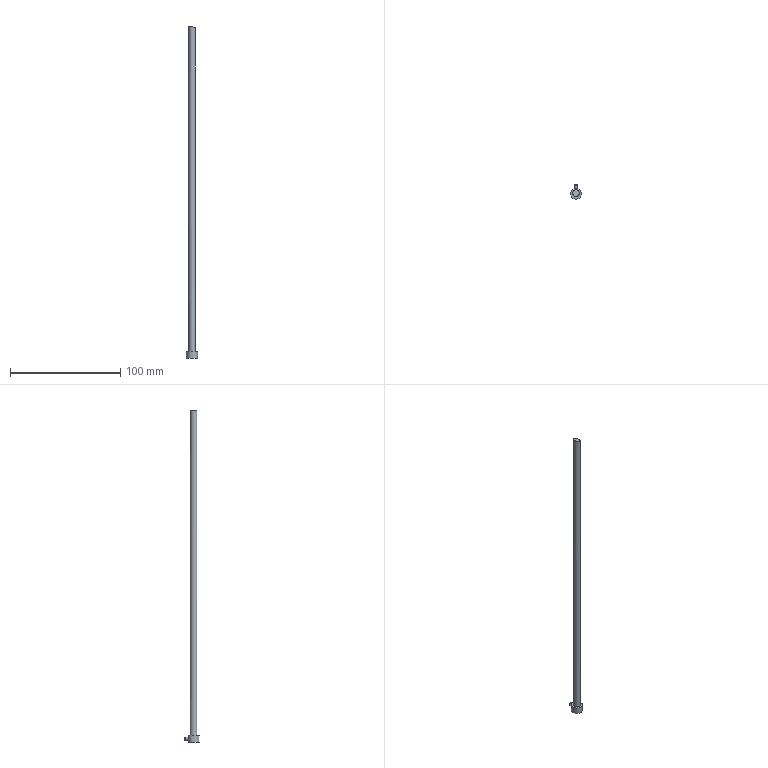Part | STEP file | E106-16-310 | 1 solid | 8 faces | box 10 x 13 x 301.324 mm | volume 8818 mm3 | cylinder 3 | plane 3 | spline 1 | cone 1 | commonest cylinder face diameters 3 x1 6 x1 10 x1